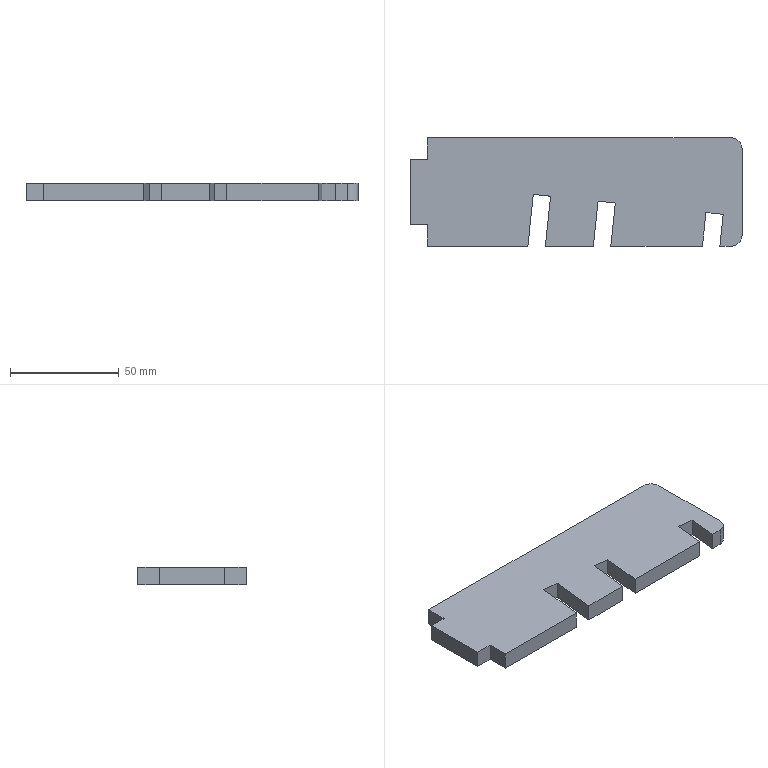Part | SolidWorks | features Fillet 1, FlatPattern 1, SMBaseFlange 1, SheetMetal 1 | 1 solid | 24 faces | box 153 x 50 x 8 mm | volume 56042 mm3 | plane 22 | cylinder 2 | commonest cylinder face diameters 10 x2
STEP:
#1=CARTESIAN_POINT('',(581.248,-4.341,0.));
#2=VERTEX_POINT('',#1);
#3=CARTESIAN_POINT('',(581.248,-14.341,0.));
#4=VERTEX_POINT('',#3);
#5=CARTESIAN_POINT('',(581.248,-4.341,0.));
#6=DIRECTION('',(0.,-1.,0.));
#7=VECTOR('',#6,1000.);
#8=LINE('',#5,#7);
#9=EDGE_CURVE('',#2,#4,#8,.T.);
#10=ORIENTED_EDGE('',*,*,#9,.F.);
#11=CARTESIAN_POINT('',(581.248,-4.341,-8.));
#12=VERTEX_POINT('',#11);
#13=CARTESIAN_POINT('',(581.248,-4.341,-8.));
#14=DIRECTION('',(0.,0.,1.));
#15=VECTOR('',#14,1000.);
#16=LINE('',#13,#15);
#17=EDGE_CURVE('',#12,#2,#16,.T.);
#18=ORIENTED_EDGE('',*,*,#17,.F.);
#19=CARTESIAN_POINT('',(581.248,-14.341,-8.));
#20=VERTEX_POINT('',#19);
#21=CARTESIAN_POINT('',(581.248,-4.341,-8.));
#22=DIRECTION('',(0.,-1.,0.));
#23=VECTOR('',#22,1000.);
#24=LINE('',#21,#23);
#25=EDGE_CURVE('',#12,#20,#24,.T.);
#26=ORIENTED_EDGE('',*,*,#25,.T.);
#27=CARTESIAN_POINT('',(581.248,-14.341,-8.));
#28=DIRECTION('',(0.,0.,1.));
#29=VECTOR('',#28,1000.);
#30=LINE('',#27,#29);
#31=EDGE_CURVE('',#20,#4,#30,.T.);
#32=ORIENTED_EDGE('',*,*,#31,.T.);
#33=EDGE_LOOP('',(#10,#18,#26,#32));
#34=FACE_OUTER_BOUND('',#33,.T.);
#35=CARTESIAN_POINT('',(581.248,-4.341,-8.));
#36=DIRECTION('',(-1.,0.,0.));
#37=DIRECTION('',(0.,0.,1.));
#38=AXIS2_PLACEMENT_3D('',#35,#36,#37);
#39=PLANE('',#38);
#40=ADVANCED_FACE('',(#34),#39,.T.);
#41=CARTESIAN_POINT('',(573.248,-4.341,0.));
#42=VERTEX_POINT('',#41);
#43=CARTESIAN_POINT('',(573.248,-4.341,0.));
#44=DIRECTION('',(1.,0.,0.));
#45=VECTOR('',#44,1000.);
#46=LINE('',#43,#45);
#47=EDGE_CURVE('',#42,#2,#46,.T.);
#48=ORIENTED_EDGE('',*,*,#47,.F.);
#49=CARTESIAN_POINT('',(573.248,-4.341,-8.));
#50=VERTEX_POINT('',#49);
#51=CARTESIAN_POINT('',(573.248,-4.341,-8.));
#52=DIRECTION('',(0.,0.,1.));
#53=VECTOR('',#52,1000.);
#54=LINE('',#51,#53);
#55=EDGE_CURVE('',#50,#42,#54,.T.);
#56=ORIENTED_EDGE('',*,*,#55,.F.);
#57=CARTESIAN_POINT('',(573.248,-4.341,-8.));
#58=DIRECTION('',(1.,0.,0.));
#59=VECTOR('',#58,1000.);
#60=LINE('',#57,#59);
#61=EDGE_CURVE('',#50,#12,#60,.T.);
#62=ORIENTED_EDGE('',*,*,#61,.T.);
#63=ORIENTED_EDGE('',*,*,#17,.T.);
#64=EDGE_LOOP('',(#48,#56,#62,#63));
#65=FACE_OUTER_BOUND('',#64,.T.);
#66=CARTESIAN_POINT('',(573.248,-4.341,-8.));
#67=DIRECTION('',(0.,-1.,0.));
#68=DIRECTION('',(0.,0.,-1.));
#69=AXIS2_PLACEMENT_3D('',#66,#67,#68);
#70=PLANE('',#69);
#71=ADVANCED_FACE('',(#65),#70,.T.);
#72=CARTESIAN_POINT('',(573.248,25.659,0.));
#73=VERTEX_POINT('',#72);
#74=CARTESIAN_POINT('',(573.248,25.659,0.));
#75=DIRECTION('',(0.,-1.,0.));
#76=VECTOR('',#75,1000.);
#77=LINE('',#74,#76);
#78=EDGE_CURVE('',#73,#42,#77,.T.);
#79=ORIENTED_EDGE('',*,*,#78,.F.);
#80=CARTESIAN_POINT('',(573.248,25.659,-8.));
#81=VERTEX_POINT('',#80);
#82=CARTESIAN_POINT('',(573.248,25.659,-8.));
#83=DIRECTION('',(0.,0.,1.));
#84=VECTOR('',#83,1000.);
#85=LINE('',#82,#84);
#86=EDGE_CURVE('',#81,#73,#85,.T.);
#87=ORIENTED_EDGE('',*,*,#86,.F.);
#88=CARTESIAN_POINT('',(573.248,25.659,-8.));
#89=DIRECTION('',(0.,-1.,0.));
#90=VECTOR('',#89,1000.);
#91=LINE('',#88,#90);
#92=EDGE_CURVE('',#81,#50,#91,.T.);
#93=ORIENTED_EDGE('',*,*,#92,.T.);
#94=ORIENTED_EDGE('',*,*,#55,.T.);
#95=EDGE_LOOP('',(#79,#87,#93,#94));
#96=FACE_OUTER_BOUND('',#95,.T.);
#97=CARTESIAN_POINT('',(573.248,25.659,-8.));
#98=DIRECTION('',(-1.,0.,0.));
#99=DIRECTION('',(0.,0.,1.));
#100=AXIS2_PLACEMENT_3D('',#97,#98,#99);
#101=PLANE('',#100);
#102=ADVANCED_FACE('',(#96),#101,.T.);
#103=CARTESIAN_POINT('',(581.248,25.659,0.));
#104=VERTEX_POINT('',#103);
#105=CARTESIAN_POINT('',(581.248,25.659,0.));
#106=DIRECTION('',(-1.,0.,0.));
#107=VECTOR('',#106,1000.);
#108=LINE('',#105,#107);
#109=EDGE_CURVE('',#104,#73,#108,.T.);
#110=ORIENTED_EDGE('',*,*,#109,.F.);
#111=CARTESIAN_POINT('',(581.248,25.659,-8.));
#112=VERTEX_POINT('',#111);
#113=CARTESIAN_POINT('',(581.248,25.659,-8.));
#114=DIRECTION('',(0.,0.,1.));
#115=VECTOR('',#114,1000.);
#116=LINE('',#113,#115);
#117=EDGE_CURVE('',#112,#104,#116,.T.);
#118=ORIENTED_EDGE('',*,*,#117,.F.);
#119=CARTESIAN_POINT('',(581.248,25.659,-8.));
#120=DIRECTION('',(-1.,0.,0.));
#121=VECTOR('',#120,1000.);
#122=LINE('',#119,#121);
#123=EDGE_CURVE('',#112,#81,#122,.T.);
#124=ORIENTED_EDGE('',*,*,#123,.T.);
#125=ORIENTED_EDGE('',*,*,#86,.T.);
#126=EDGE_LOOP('',(#110,#118,#124,#125));
#127=FACE_OUTER_BOUND('',#126,.T.);
#128=CARTESIAN_POINT('',(581.248,25.659,-8.));
#129=DIRECTION('',(0.,1.,0.));
#130=DIRECTION('',(0.,0.,1.));
#131=AXIS2_PLACEMENT_3D('',#128,#129,#130);
#132=PLANE('',#131);
#133=ADVANCED_FACE('',(#127),#132,.T.);
#134=CARTESIAN_POINT('',(581.248,35.659,0.));
#135=VERTEX_POINT('',#134);
#136=CARTESIAN_POINT('',(581.248,35.659,0.));
#137=DIRECTION('',(0.,-1.,0.));
#138=VECTOR('',#137,1000.);
#139=LINE('',#136,#138);
#140=EDGE_CURVE('',#135,#104,#139,.T.);
#141=ORIENTED_EDGE('',*,*,#140,.F.);
#142=CARTESIAN_POINT('',(581.248,35.659,-8.));
#143=VERTEX_POINT('',#142);
#144=CARTESIAN_POINT('',(581.248,35.659,-8.));
#145=DIRECTION('',(0.,0.,1.));
#146=VECTOR('',#145,1000.);
#147=LINE('',#144,#146);
#148=EDGE_CURVE('',#143,#135,#147,.T.);
#149=ORIENTED_EDGE('',*,*,#148,.F.);
#150=CARTESIAN_POINT('',(581.248,35.659,-8.));
#151=DIRECTION('',(0.,-1.,0.));
#152=VECTOR('',#151,1000.);
#153=LINE('',#150,#152);
#154=EDGE_CURVE('',#143,#112,#153,.T.);
#155=ORIENTED_EDGE('',*,*,#154,.T.);
#156=ORIENTED_EDGE('',*,*,#117,.T.);
#157=EDGE_LOOP('',(#141,#149,#155,#156));
#158=FACE_OUTER_BOUND('',#157,.T.);
#159=CARTESIAN_POINT('',(581.248,35.659,-8.));
#160=DIRECTION('',(-1.,0.,0.));
#161=DIRECTION('',(0.,0.,1.));
#162=AXIS2_PLACEMENT_3D('',#159,#160,#161);
#163=PLANE('',#162);
#164=ADVANCED_FACE('',(#158),#163,.T.);
#165=CARTESIAN_POINT('',(721.248,35.659,0.));
#166=VERTEX_POINT('',#165);
#167=CARTESIAN_POINT('',(726.248,35.659,0.));
#168=DIRECTION('',(-1.,0.,0.));
#169=VECTOR('',#168,1000.);
#170=LINE('',#167,#169);
#171=EDGE_CURVE('',#166,#135,#170,.T.);
#172=ORIENTED_EDGE('',*,*,#171,.F.);
#173=CARTESIAN_POINT('',(721.248,35.659,-8.));
#174=VERTEX_POINT('',#173);
#175=CARTESIAN_POINT('',(721.248,35.659,-8.));
#176=DIRECTION('',(0.,0.,-1.));
#177=VECTOR('',#176,1000.);
#178=LINE('',#175,#177);
#179=EDGE_CURVE('',#166,#174,#178,.T.);
#180=ORIENTED_EDGE('',*,*,#179,.T.);
#181=CARTESIAN_POINT('',(726.248,35.659,-8.));
#182=DIRECTION('',(-1.,0.,0.));
#183=VECTOR('',#182,1000.);
#184=LINE('',#181,#183);
#185=EDGE_CURVE('',#174,#143,#184,.T.);
#186=ORIENTED_EDGE('',*,*,#185,.T.);
#187=ORIENTED_EDGE('',*,*,#148,.T.);
#188=EDGE_LOOP('',(#172,#180,#186,#187));
#189=FACE_OUTER_BOUND('',#188,.T.);
#190=CARTESIAN_POINT('',(726.248,35.659,-8.));
#191=DIRECTION('',(0.,1.,0.));
#192=DIRECTION('',(0.,0.,1.));
#193=AXIS2_PLACEMENT_3D('',#190,#191,#192);
#194=PLANE('',#193);
#195=ADVANCED_FACE('',(#189),#194,.T.);
#196=CARTESIAN_POINT('',(726.248,-9.341,0.));
#197=VERTEX_POINT('',#196);
#198=CARTESIAN_POINT('',(726.248,30.659,0.));
#199=VERTEX_POINT('',#198);
#200=CARTESIAN_POINT('',(726.248,-14.341,0.));
#201=DIRECTION('',(0.,1.,0.));
#202=VECTOR('',#201,1000.);
#203=LINE('',#200,#202);
#204=EDGE_CURVE('',#197,#199,#203,.T.);
#205=ORIENTED_EDGE('',*,*,#204,.F.);
#206=CARTESIAN_POINT('',(726.248,-9.341,-8.));
#207=VERTEX_POINT('',#206);
#208=CARTESIAN_POINT('',(726.248,-9.341,-8.));
#209=DIRECTION('',(0.,0.,-1.));
#210=VECTOR('',#209,1000.);
#211=LINE('',#208,#210);
#212=EDGE_CURVE('',#197,#207,#211,.T.);
#213=ORIENTED_EDGE('',*,*,#212,.T.);
#214=CARTESIAN_POINT('',(726.248,30.659,-8.));
#215=VERTEX_POINT('',#214);
#216=CARTESIAN_POINT('',(726.248,-14.341,-8.));
#217=DIRECTION('',(0.,1.,0.));
#218=VECTOR('',#217,1000.);
#219=LINE('',#216,#218);
#220=EDGE_CURVE('',#207,#215,#219,.T.);
#221=ORIENTED_EDGE('',*,*,#220,.T.);
#222=CARTESIAN_POINT('',(726.248,30.659,-8.));
#223=DIRECTION('',(0.,0.,1.));
#224=VECTOR('',#223,1000.);
#225=LINE('',#222,#224);
#226=EDGE_CURVE('',#215,#199,#225,.T.);
#227=ORIENTED_EDGE('',*,*,#226,.T.);
#228=EDGE_LOOP('',(#205,#213,#221,#227));
#229=FACE_OUTER_BOUND('',#228,.T.);
#230=CARTESIAN_POINT('',(726.248,-14.341,-8.));
#231=DIRECTION('',(1.,0.,0.));
#232=DIRECTION('',(0.,0.,-1.));
#233=AXIS2_PLACEMENT_3D('',#230,#231,#232);
#234=PLANE('',#233);
#235=ADVANCED_FACE('',(#229),#234,.T.);
#236=CARTESIAN_POINT('',(716.041,-14.341,-8.));
#237=VERTEX_POINT('',#236);
#238=CARTESIAN_POINT('',(721.248,-14.341,-8.));
#239=VERTEX_POINT('',#238);
#240=CARTESIAN_POINT('',(716.041,-14.341,-8.));
#241=DIRECTION('',(1.,0.,0.));
#242=VECTOR('',#241,1000.);
#243=LINE('',#240,#242);
#244=EDGE_CURVE('',#237,#239,#243,.T.);
#245=ORIENTED_EDGE('',*,*,#244,.T.);
#246=CARTESIAN_POINT('',(721.248,-14.341,0.));
#247=VERTEX_POINT('',#246);
#248=CARTESIAN_POINT('',(721.248,-14.341,-8.));
#249=DIRECTION('',(0.,0.,1.));
#250=VECTOR('',#249,1000.);
#251=LINE('',#248,#250);
#252=EDGE_CURVE('',#239,#247,#251,.T.);
#253=ORIENTED_EDGE('',*,*,#252,.T.);
#254=CARTESIAN_POINT('',(716.041,-14.341,0.));
#255=VERTEX_POINT('',#254);
#256=CARTESIAN_POINT('',(716.041,-14.341,0.));
#257=DIRECTION('',(1.,0.,0.));
#258=VECTOR('',#257,1000.);
#259=LINE('',#256,#258);
#260=EDGE_CURVE('',#255,#247,#259,.T.);
#261=ORIENTED_EDGE('',*,*,#260,.F.);
#262=CARTESIAN_POINT('',(716.041,-14.341,-8.));
#263=DIRECTION('',(0.,0.,1.));
#264=VECTOR('',#263,1000.);
#265=LINE('',#262,#264);
#266=EDGE_CURVE('',#237,#255,#265,.T.);
#267=ORIENTED_EDGE('',*,*,#266,.F.);
#268=EDGE_LOOP('',(#245,#253,#261,#267));
#269=FACE_OUTER_BOUND('',#268,.T.);
#270=CARTESIAN_POINT('',(716.041,-14.341,-8.));
#271=DIRECTION('',(0.,-1.,0.));
#272=DIRECTION('',(0.,0.,-1.));
#273=AXIS2_PLACEMENT_3D('',#270,#271,#272);
#274=PLANE('',#273);
#275=ADVANCED_FACE('',(#269),#274,.T.);
#276=CARTESIAN_POINT('',(717.584,0.3623,0.));
#277=VERTEX_POINT('',#276);
#278=CARTESIAN_POINT('',(717.584,0.3623,0.));
#279=DIRECTION('',(-0.1044,-0.9945,0.));
#280=VECTOR('',#279,1000.);
#281=LINE('',#278,#280);
#282=EDGE_CURVE('',#277,#255,#281,.T.);
#283=ORIENTED_EDGE('',*,*,#282,.F.);
#284=CARTESIAN_POINT('',(717.584,0.3623,-8.));
#285=VERTEX_POINT('',#284);
#286=CARTESIAN_POINT('',(717.584,0.3623,-8.));
#287=DIRECTION('',(0.,0.,1.));
#288=VECTOR('',#287,1000.);
#289=LINE('',#286,#288);
#290=EDGE_CURVE('',#285,#277,#289,.T.);
#291=ORIENTED_EDGE('',*,*,#290,.F.);
#292=CARTESIAN_POINT('',(717.584,0.3623,-8.));
#293=DIRECTION('',(-0.1044,-0.9945,0.));
#294=VECTOR('',#293,1000.);
#295=LINE('',#292,#294);
#296=EDGE_CURVE('',#285,#237,#295,.T.);
#297=ORIENTED_EDGE('',*,*,#296,.T.);
#298=ORIENTED_EDGE('',*,*,#266,.T.);
#299=EDGE_LOOP('',(#283,#291,#297,#298));
#300=FACE_OUTER_BOUND('',#299,.T.);
#301=CARTESIAN_POINT('',(717.584,0.3623,-8.));
#302=DIRECTION('',(-0.9945,0.1044,0.));
#303=DIRECTION('',(-0.1044,-0.9945,0.));
#304=AXIS2_PLACEMENT_3D('',#301,#302,#303);
#305=PLANE('',#304);
#306=ADVANCED_FACE('',(#300),#305,.T.);
#307=CARTESIAN_POINT('',(709.628,1.198,0.));
#308=VERTEX_POINT('',#307);
#309=CARTESIAN_POINT('',(717.584,0.3623,0.));
#310=DIRECTION('',(0.9945,-0.1044,0.));
#311=VECTOR('',#310,1000.);
#312=LINE('',#309,#311);
#313=EDGE_CURVE('',#308,#277,#312,.T.);
#314=ORIENTED_EDGE('',*,*,#313,.F.);
#315=CARTESIAN_POINT('',(709.628,1.198,-8.));
#316=VERTEX_POINT('',#315);
#317=CARTESIAN_POINT('',(709.628,1.198,-8.));
#318=DIRECTION('',(0.,0.,1.));
#319=VECTOR('',#318,1000.);
#320=LINE('',#317,#319);
#321=EDGE_CURVE('',#316,#308,#320,.T.);
#322=ORIENTED_EDGE('',*,*,#321,.F.);
#323=CARTESIAN_POINT('',(717.584,0.3623,-8.));
#324=DIRECTION('',(0.9945,-0.1044,0.));
#325=VECTOR('',#324,1000.);
#326=LINE('',#323,#325);
#327=EDGE_CURVE('',#316,#285,#326,.T.);
#328=ORIENTED_EDGE('',*,*,#327,.T.);
#329=ORIENTED_EDGE('',*,*,#290,.T.);
#330=EDGE_LOOP('',(#314,#322,#328,#329));
#331=FACE_OUTER_BOUND('',#330,.T.);
#332=CARTESIAN_POINT('',(717.584,0.3623,-8.));
#333=DIRECTION('',(-0.1044,-0.9945,0.));
#334=DIRECTION('',(0.9945,-0.1044,0.));
#335=AXIS2_PLACEMENT_3D('',#332,#333,#334);
#336=PLANE('',#335);
#337=ADVANCED_FACE('',(#331),#336,.T.);
#338=CARTESIAN_POINT('',(707.997,-14.341,0.));
#339=VERTEX_POINT('',#338);
#340=CARTESIAN_POINT('',(709.628,1.198,0.));
#341=DIRECTION('',(0.1044,0.9945,0.));
#342=VECTOR('',#341,1000.);
#343=LINE('',#340,#342);
#344=EDGE_CURVE('',#339,#308,#343,.T.);
#345=ORIENTED_EDGE('',*,*,#344,.F.);
#346=CARTESIAN_POINT('',(707.997,-14.341,-8.));
#347=VERTEX_POINT('',#346);
#348=CARTESIAN_POINT('',(707.997,-14.341,-8.));
#349=DIRECTION('',(0.,0.,1.));
#350=VECTOR('',#349,1000.);
#351=LINE('',#348,#350);
#352=EDGE_CURVE('',#347,#339,#351,.T.);
#353=ORIENTED_EDGE('',*,*,#352,.F.);
#354=CARTESIAN_POINT('',(709.628,1.198,-8.));
#355=DIRECTION('',(0.1044,0.9945,0.));
#356=VECTOR('',#355,1000.);
#357=LINE('',#354,#356);
#358=EDGE_CURVE('',#347,#316,#357,.T.);
#359=ORIENTED_EDGE('',*,*,#358,.T.);
#360=ORIENTED_EDGE('',*,*,#321,.T.);
#361=EDGE_LOOP('',(#345,#353,#359,#360));
#362=FACE_OUTER_BOUND('',#361,.T.);
#363=CARTESIAN_POINT('',(709.628,1.198,-8.));
#364=DIRECTION('',(0.9945,-0.1044,0.));
#365=DIRECTION('',(0.1044,0.9945,0.));
#366=AXIS2_PLACEMENT_3D('',#363,#364,#365);
#367=PLANE('',#366);
#368=ADVANCED_FACE('',(#362),#367,.T.);
#369=CARTESIAN_POINT('',(665.766,-14.341,0.));
#370=VERTEX_POINT('',#369);
#371=CARTESIAN_POINT('',(665.766,-14.341,0.));
#372=DIRECTION('',(1.,0.,0.));
#373=VECTOR('',#372,1000.);
#374=LINE('',#371,#373);
#375=EDGE_CURVE('',#370,#339,#374,.T.);
#376=ORIENTED_EDGE('',*,*,#375,.F.);
#377=CARTESIAN_POINT('',(665.766,-14.341,-8.));
#378=VERTEX_POINT('',#377);
#379=CARTESIAN_POINT('',(665.766,-14.341,-8.));
#380=DIRECTION('',(0.,0.,1.));
#381=VECTOR('',#380,1000.);
#382=LINE('',#379,#381);
#383=EDGE_CURVE('',#378,#370,#382,.T.);
#384=ORIENTED_EDGE('',*,*,#383,.F.);
#385=CARTESIAN_POINT('',(665.766,-14.341,-8.));
#386=DIRECTION('',(1.,0.,0.));
#387=VECTOR('',#386,1000.);
#388=LINE('',#385,#387);
#389=EDGE_CURVE('',#378,#347,#388,.T.);
#390=ORIENTED_EDGE('',*,*,#389,.T.);
#391=ORIENTED_EDGE('',*,*,#352,.T.);
#392=EDGE_LOOP('',(#376,#384,#390,#391));
#393=FACE_OUTER_BOUND('',#392,.T.);
#394=CARTESIAN_POINT('',(665.766,-14.341,-8.));
#395=DIRECTION('',(0.,-1.,0.));
#396=DIRECTION('',(1.,0.,0.));
#397=AXIS2_PLACEMENT_3D('',#394,#395,#396);
#398=PLANE('',#397);
#399=ADVANCED_FACE('',(#393),#398,.T.);
#400=CARTESIAN_POINT('',(667.858,5.583,0.));
#401=VERTEX_POINT('',#400);
#402=CARTESIAN_POINT('',(667.858,5.583,0.));
#403=DIRECTION('',(-0.1044,-0.9945,0.));
#404=VECTOR('',#403,1000.);
#405=LINE('',#402,#404);
#406=EDGE_CURVE('',#401,#370,#405,.T.);
#407=ORIENTED_EDGE('',*,*,#406,.F.);
#408=CARTESIAN_POINT('',(667.858,5.583,-8.));
#409=VERTEX_POINT('',#408);
#410=CARTESIAN_POINT('',(667.858,5.583,-8.));
#411=DIRECTION('',(0.,0.,1.));
#412=VECTOR('',#411,1000.);
#413=LINE('',#410,#412);
#414=EDGE_CURVE('',#409,#401,#413,.T.);
#415=ORIENTED_EDGE('',*,*,#414,.F.);
#416=CARTESIAN_POINT('',(667.858,5.583,-8.));
#417=DIRECTION('',(-0.1044,-0.9945,0.));
#418=VECTOR('',#417,1000.);
#419=LINE('',#416,#418);
#420=EDGE_CURVE('',#409,#378,#419,.T.);
#421=ORIENTED_EDGE('',*,*,#420,.T.);
#422=ORIENTED_EDGE('',*,*,#383,.T.);
#423=EDGE_LOOP('',(#407,#415,#421,#422));
#424=FACE_OUTER_BOUND('',#423,.T.);
#425=CARTESIAN_POINT('',(667.858,5.583,-8.));
#426=DIRECTION('',(-0.9945,0.1044,0.));
#427=DIRECTION('',(-0.1044,-0.9945,0.));
#428=AXIS2_PLACEMENT_3D('',#425,#426,#427);
#429=PLANE('',#428);
#430=ADVANCED_FACE('',(#424),#429,.T.);
#431=CARTESIAN_POINT('',(659.901,6.418,0.));
#432=VERTEX_POINT('',#431);
#433=CARTESIAN_POINT('',(667.858,5.583,0.));
#434=DIRECTION('',(0.9945,-0.1044,0.));
#435=VECTOR('',#434,1000.);
#436=LINE('',#433,#435);
#437=EDGE_CURVE('',#432,#401,#436,.T.);
#438=ORIENTED_EDGE('',*,*,#437,.F.);
#439=CARTESIAN_POINT('',(659.901,6.418,-8.));
#440=VERTEX_POINT('',#439);
#441=CARTESIAN_POINT('',(659.901,6.418,-8.));
#442=DIRECTION('',(0.,0.,1.));
#443=VECTOR('',#442,1000.);
#444=LINE('',#441,#443);
#445=EDGE_CURVE('',#440,#432,#444,.T.);
#446=ORIENTED_EDGE('',*,*,#445,.F.);
#447=CARTESIAN_POINT('',(667.858,5.583,-8.));
#448=DIRECTION('',(0.9945,-0.1044,0.));
#449=VECTOR('',#448,1000.);
#450=LINE('',#447,#449);
#451=EDGE_CURVE('',#440,#409,#450,.T.);
#452=ORIENTED_EDGE('',*,*,#451,.T.);
#453=ORIENTED_EDGE('',*,*,#414,.T.);
#454=EDGE_LOOP('',(#438,#446,#452,#453));
#455=FACE_OUTER_BOUND('',#454,.T.);
#456=CARTESIAN_POINT('',(667.858,5.583,-8.));
#457=DIRECTION('',(-0.1044,-0.9945,0.));
#458=DIRECTION('',(0.9945,-0.1044,0.));
#459=AXIS2_PLACEMENT_3D('',#456,#457,#458);
#460=PLANE('',#459);
#461=ADVANCED_FACE('',(#455),#460,.T.);
#462=CARTESIAN_POINT('',(657.722,-14.341,0.));
#463=VERTEX_POINT('',#462);
#464=CARTESIAN_POINT('',(659.901,6.418,0.));
#465=DIRECTION('',(0.1044,0.9945,0.));
#466=VECTOR('',#465,1000.);
#467=LINE('',#464,#466);
#468=EDGE_CURVE('',#463,#432,#467,.T.);
#469=ORIENTED_EDGE('',*,*,#468,.F.);
#470=CARTESIAN_POINT('',(657.722,-14.341,-8.));
#471=VERTEX_POINT('',#470);
#472=CARTESIAN_POINT('',(657.722,-14.341,-8.));
#473=DIRECTION('',(0.,0.,1.));
#474=VECTOR('',#473,1000.);
#475=LINE('',#472,#474);
#476=EDGE_CURVE('',#471,#463,#475,.T.);
#477=ORIENTED_EDGE('',*,*,#476,.F.);
#478=CARTESIAN_POINT('',(659.901,6.418,-8.));
#479=DIRECTION('',(0.1044,0.9945,0.));
#480=VECTOR('',#479,1000.);
#481=LINE('',#478,#480);
#482=EDGE_CURVE('',#471,#440,#481,.T.);
#483=ORIENTED_EDGE('',*,*,#482,.T.);
#484=ORIENTED_EDGE('',*,*,#445,.T.);
#485=EDGE_LOOP('',(#469,#477,#483,#484));
#486=FACE_OUTER_BOUND('',#485,.T.);
#487=CARTESIAN_POINT('',(659.901,6.418,-8.));
#488=DIRECTION('',(0.9945,-0.1044,0.));
#489=DIRECTION('',(0.1044,0.9945,0.));
#490=AXIS2_PLACEMENT_3D('',#487,#488,#489);
#491=PLANE('',#490);
#492=ADVANCED_FACE('',(#486),#491,.T.);
#493=CARTESIAN_POINT('',(635.601,-14.341,0.));
#494=VERTEX_POINT('',#493);
#495=CARTESIAN_POINT('',(635.601,-14.341,0.));
#496=DIRECTION('',(1.,0.,0.));
#497=VECTOR('',#496,1000.);
#498=LINE('',#495,#497);
#499=EDGE_CURVE('',#494,#463,#498,.T.);
#500=ORIENTED_EDGE('',*,*,#499,.F.);
#501=CARTESIAN_POINT('',(635.601,-14.341,-8.));
#502=VERTEX_POINT('',#501);
#503=CARTESIAN_POINT('',(635.601,-14.341,-8.));
#504=DIRECTION('',(0.,0.,1.));
#505=VECTOR('',#504,1000.);
#506=LINE('',#503,#505);
#507=EDGE_CURVE('',#502,#494,#506,.T.);
#508=ORIENTED_EDGE('',*,*,#507,.F.);
#509=CARTESIAN_POINT('',(635.601,-14.341,-8.));
#510=DIRECTION('',(1.,0.,0.));
#511=VECTOR('',#510,1000.);
#512=LINE('',#509,#511);
#513=EDGE_CURVE('',#502,#471,#512,.T.);
#514=ORIENTED_EDGE('',*,*,#513,.T.);
#515=ORIENTED_EDGE('',*,*,#476,.T.);
#516=EDGE_LOOP('',(#500,#508,#514,#515));
#517=FACE_OUTER_BOUND('',#516,.T.);
#518=CARTESIAN_POINT('',(635.601,-14.341,-8.));
#519=DIRECTION('',(0.,-1.,0.));
#520=DIRECTION('',(0.,0.,-1.));
#521=AXIS2_PLACEMENT_3D('',#518,#519,#520);
#522=PLANE('',#521);
#523=ADVANCED_FACE('',(#517),#522,.T.);
#524=CARTESIAN_POINT('',(638.022,8.715,0.));
#525=VERTEX_POINT('',#524);
#526=CARTESIAN_POINT('',(638.022,8.715,0.));
#527=DIRECTION('',(-0.1044,-0.9945,0.));
#528=VECTOR('',#527,1000.);
#529=LINE('',#526,#528);
#530=EDGE_CURVE('',#525,#494,#529,.T.);
#531=ORIENTED_EDGE('',*,*,#530,.F.);
#532=CARTESIAN_POINT('',(638.022,8.715,-8.));
#533=VERTEX_POINT('',#532);
#534=CARTESIAN_POINT('',(638.022,8.715,-8.));
#535=DIRECTION('',(0.,0.,1.));
#536=VECTOR('',#535,1000.);
#537=LINE('',#534,#536);
#538=EDGE_CURVE('',#533,#525,#537,.T.);
#539=ORIENTED_EDGE('',*,*,#538,.F.);
#540=CARTESIAN_POINT('',(638.022,8.715,-8.));
#541=DIRECTION('',(-0.1044,-0.9945,0.));
#542=VECTOR('',#541,1000.);
#543=LINE('',#540,#542);
#544=EDGE_CURVE('',#533,#502,#543,.T.);
#545=ORIENTED_EDGE('',*,*,#544,.T.);
#546=ORIENTED_EDGE('',*,*,#507,.T.);
#547=EDGE_LOOP('',(#531,#539,#545,#546));
#548=FACE_OUTER_BOUND('',#547,.T.);
#549=CARTESIAN_POINT('',(638.022,8.715,-8.));
#550=DIRECTION('',(-0.9945,0.1044,0.));
#551=DIRECTION('',(-0.1044,-0.9945,0.));
#552=AXIS2_PLACEMENT_3D('',#549,#550,#551);
#553=PLANE('',#552);
#554=ADVANCED_FACE('',(#548),#553,.T.);
#555=CARTESIAN_POINT('',(630.065,9.551,0.));
#556=VERTEX_POINT('',#555);
#557=CARTESIAN_POINT('',(638.022,8.715,0.));
#558=DIRECTION('',(0.9945,-0.1044,0.));
#559=VECTOR('',#558,1000.);
#560=LINE('',#557,#559);
#561=EDGE_CURVE('',#556,#525,#560,.T.);
#562=ORIENTED_EDGE('',*,*,#561,.F.);
#563=CARTESIAN_POINT('',(630.065,9.551,-8.));
#564=VERTEX_POINT('',#563);
#565=CARTESIAN_POINT('',(630.065,9.551,-8.));
#566=DIRECTION('',(0.,0.,1.));
#567=VECTOR('',#566,1000.);
#568=LINE('',#565,#567);
#569=EDGE_CURVE('',#564,#556,#568,.T.);
#570=ORIENTED_EDGE('',*,*,#569,.F.);
#571=CARTESIAN_POINT('',(638.022,8.715,-8.));
#572=DIRECTION('',(0.9945,-0.1044,0.));
#573=VECTOR('',#572,1000.);
#574=LINE('',#571,#573);
#575=EDGE_CURVE('',#564,#533,#574,.T.);
#576=ORIENTED_EDGE('',*,*,#575,.T.);
#577=ORIENTED_EDGE('',*,*,#538,.T.);
#578=EDGE_LOOP('',(#562,#570,#576,#577));
#579=FACE_OUTER_BOUND('',#578,.T.);
#580=CARTESIAN_POINT('',(638.022,8.715,-8.));
#581=DIRECTION('',(-0.1044,-0.9945,0.));
#582=DIRECTION('',(0.9945,-0.1044,0.));
#583=AXIS2_PLACEMENT_3D('',#580,#581,#582);
#584=PLANE('',#583);
#585=ADVANCED_FACE('',(#579),#584,.T.);
#586=CARTESIAN_POINT('',(627.557,-14.341,0.));
#587=VERTEX_POINT('',#586);
#588=CARTESIAN_POINT('',(630.065,9.551,0.));
#589=DIRECTION('',(0.1044,0.9945,0.));
#590=VECTOR('',#589,1000.);
#591=LINE('',#588,#590);
#592=EDGE_CURVE('',#587,#556,#591,.T.);
#593=ORIENTED_EDGE('',*,*,#592,.F.);
#594=CARTESIAN_POINT('',(627.557,-14.341,-8.));
#595=VERTEX_POINT('',#594);
#596=CARTESIAN_POINT('',(627.557,-14.341,-8.));
#597=DIRECTION('',(0.,0.,1.));
#598=VECTOR('',#597,1000.);
#599=LINE('',#596,#598);
#600=EDGE_CURVE('',#595,#587,#599,.T.);
#601=ORIENTED_EDGE('',*,*,#600,.F.);
#602=CARTESIAN_POINT('',(630.065,9.551,-8.));
#603=DIRECTION('',(0.1044,0.9945,0.));
#604=VECTOR('',#603,1000.);
#605=LINE('',#602,#604);
#606=EDGE_CURVE('',#595,#564,#605,.T.);
#607=ORIENTED_EDGE('',*,*,#606,.T.);
#608=ORIENTED_EDGE('',*,*,#569,.T.);
#609=EDGE_LOOP('',(#593,#601,#607,#608));
#610=FACE_OUTER_BOUND('',#609,.T.);
#611=CARTESIAN_POINT('',(630.065,9.551,-8.));
#612=DIRECTION('',(0.9945,-0.1044,0.));
#613=DIRECTION('',(0.1044,0.9945,0.));
#614=AXIS2_PLACEMENT_3D('',#611,#612,#613);
#615=PLANE('',#614);
#616=ADVANCED_FACE('',(#610),#615,.T.);
#617=CARTESIAN_POINT('',(581.248,-14.341,0.));
#618=DIRECTION('',(1.,0.,0.));
#619=VECTOR('',#618,1000.);
#620=LINE('',#617,#619);
#621=EDGE_CURVE('',#4,#587,#620,.T.);
#622=ORIENTED_EDGE('',*,*,#621,.F.);
#623=ORIENTED_EDGE('',*,*,#31,.F.);
#624=CARTESIAN_POINT('',(581.248,-14.341,-8.));
#625=DIRECTION('',(1.,0.,0.));
#626=VECTOR('',#625,1000.);
#627=LINE('',#624,#626);
#628=EDGE_CURVE('',#20,#595,#627,.T.);
#629=ORIENTED_EDGE('',*,*,#628,.T.);
#630=ORIENTED_EDGE('',*,*,#600,.T.);
#631=EDGE_LOOP('',(#622,#623,#629,#630));
#632=FACE_OUTER_BOUND('',#631,.T.);
#633=CARTESIAN_POINT('',(581.248,-14.341,-8.));
#634=DIRECTION('',(0.,-1.,0.));
#635=DIRECTION('',(1.,0.,0.));
#636=AXIS2_PLACEMENT_3D('',#633,#634,#635);
#637=PLANE('',#636);
#638=ADVANCED_FACE('',(#632),#637,.T.);
#639=ORIENTED_EDGE('',*,*,#220,.F.);
#640=CARTESIAN_POINT('',(721.248,-9.341,-8.));
#641=DIRECTION('',(0.,0.,-1.));
#642=DIRECTION('',(1.,0.,0.));
#643=AXIS2_PLACEMENT_3D('',#640,#641,#642);
#644=CIRCLE('',#643,5.);
#645=EDGE_CURVE('',#207,#239,#644,.T.);
#646=ORIENTED_EDGE('',*,*,#645,.T.);
#647=ORIENTED_EDGE('',*,*,#244,.F.);
#648=ORIENTED_EDGE('',*,*,#296,.F.);
#649=ORIENTED_EDGE('',*,*,#327,.F.);
#650=ORIENTED_EDGE('',*,*,#358,.F.);
#651=ORIENTED_EDGE('',*,*,#389,.F.);
#652=ORIENTED_EDGE('',*,*,#420,.F.);
#653=ORIENTED_EDGE('',*,*,#451,.F.);
#654=ORIENTED_EDGE('',*,*,#482,.F.);
#655=ORIENTED_EDGE('',*,*,#513,.F.);
#656=ORIENTED_EDGE('',*,*,#544,.F.);
#657=ORIENTED_EDGE('',*,*,#575,.F.);
#658=ORIENTED_EDGE('',*,*,#606,.F.);
#659=ORIENTED_EDGE('',*,*,#628,.F.);
#660=ORIENTED_EDGE('',*,*,#25,.F.);
#661=ORIENTED_EDGE('',*,*,#61,.F.);
#662=ORIENTED_EDGE('',*,*,#92,.F.);
#663=ORIENTED_EDGE('',*,*,#123,.F.);
#664=ORIENTED_EDGE('',*,*,#154,.F.);
#665=ORIENTED_EDGE('',*,*,#185,.F.);
#666=CARTESIAN_POINT('',(721.248,30.659,-8.));
#667=DIRECTION('',(0.,0.,-1.));
#668=DIRECTION('',(1.,0.,0.));
#669=AXIS2_PLACEMENT_3D('',#666,#667,#668);
#670=CIRCLE('',#669,5.);
#671=EDGE_CURVE('',#174,#215,#670,.T.);
#672=ORIENTED_EDGE('',*,*,#671,.T.);
#673=EDGE_LOOP('',(#639,#646,#647,#648,#649,#650,#651,#652,#653,#654,#655,#656,#657,#658,#659,#660,#661,#662,#663,#664,#665,#672));
#674=FACE_OUTER_BOUND('',#673,.T.);
#675=CARTESIAN_POINT('',(0.,0.,-8.));
#676=DIRECTION('',(0.,0.,1.));
#677=DIRECTION('',(1.,0.,0.));
#678=AXIS2_PLACEMENT_3D('',#675,#676,#677);
#679=PLANE('',#678);
#680=ADVANCED_FACE('',(#674),#679,.F.);
#681=ORIENTED_EDGE('',*,*,#260,.T.);
#682=CARTESIAN_POINT('',(721.248,-9.341,0.));
#683=DIRECTION('',(0.,0.,1.));
#684=DIRECTION('',(1.,0.,0.));
#685=AXIS2_PLACEMENT_3D('',#682,#683,#684);
#686=CIRCLE('',#685,5.);
#687=EDGE_CURVE('',#247,#197,#686,.T.);
#688=ORIENTED_EDGE('',*,*,#687,.T.);
#689=ORIENTED_EDGE('',*,*,#204,.T.);
#690=CARTESIAN_POINT('',(721.248,30.659,0.));
#691=DIRECTION('',(0.,0.,1.));
#692=DIRECTION('',(1.,0.,0.));
#693=AXIS2_PLACEMENT_3D('',#690,#691,#692);
#694=CIRCLE('',#693,5.);
#695=EDGE_CURVE('',#199,#166,#694,.T.);
#696=ORIENTED_EDGE('',*,*,#695,.T.);
#697=ORIENTED_EDGE('',*,*,#171,.T.);
#698=ORIENTED_EDGE('',*,*,#140,.T.);
#699=ORIENTED_EDGE('',*,*,#109,.T.);
#700=ORIENTED_EDGE('',*,*,#78,.T.);
#701=ORIENTED_EDGE('',*,*,#47,.T.);
#702=ORIENTED_EDGE('',*,*,#9,.T.);
#703=ORIENTED_EDGE('',*,*,#621,.T.);
#704=ORIENTED_EDGE('',*,*,#592,.T.);
#705=ORIENTED_EDGE('',*,*,#561,.T.);
#706=ORIENTED_EDGE('',*,*,#530,.T.);
#707=ORIENTED_EDGE('',*,*,#499,.T.);
#708=ORIENTED_EDGE('',*,*,#468,.T.);
#709=ORIENTED_EDGE('',*,*,#437,.T.);
#710=ORIENTED_EDGE('',*,*,#406,.T.);
#711=ORIENTED_EDGE('',*,*,#375,.T.);
#712=ORIENTED_EDGE('',*,*,#344,.T.);
#713=ORIENTED_EDGE('',*,*,#313,.T.);
#714=ORIENTED_EDGE('',*,*,#282,.T.);
#715=EDGE_LOOP('',(#681,#688,#689,#696,#697,#698,#699,#700,#701,#702,#703,#704,#705,#706,#707,#708,#709,#710,#711,#712,#713,#714));
#716=FACE_OUTER_BOUND('',#715,.T.);
#717=CARTESIAN_POINT('',(0.,0.,0.));
#718=DIRECTION('',(0.,0.,1.));
#719=DIRECTION('',(1.,0.,0.));
#720=AXIS2_PLACEMENT_3D('',#717,#718,#719);
#721=PLANE('',#720);
#722=ADVANCED_FACE('',(#716),#721,.T.);
#723=ORIENTED_EDGE('',*,*,#645,.F.);
#724=ORIENTED_EDGE('',*,*,#212,.F.);
#725=ORIENTED_EDGE('',*,*,#687,.F.);
#726=ORIENTED_EDGE('',*,*,#252,.F.);
#727=EDGE_LOOP('',(#723,#724,#725,#726));
#728=FACE_OUTER_BOUND('',#727,.T.);
#729=CARTESIAN_POINT('',(721.248,-9.341,-8.));
#730=DIRECTION('',(0.,0.,1.));
#731=DIRECTION('',(1.,0.,0.));
#732=AXIS2_PLACEMENT_3D('',#729,#730,#731);
#733=CYLINDRICAL_SURFACE('',#732,5.);
#734=ADVANCED_FACE('',(#728),#733,.T.);
#735=ORIENTED_EDGE('',*,*,#671,.F.);
#736=ORIENTED_EDGE('',*,*,#179,.F.);
#737=ORIENTED_EDGE('',*,*,#695,.F.);
#738=ORIENTED_EDGE('',*,*,#226,.F.);
#739=EDGE_LOOP('',(#735,#736,#737,#738));
#740=FACE_OUTER_BOUND('',#739,.T.);
#741=CARTESIAN_POINT('',(721.248,30.659,-8.));
#742=DIRECTION('',(0.,0.,1.));
#743=DIRECTION('',(1.,0.,0.));
#744=AXIS2_PLACEMENT_3D('',#741,#742,#743);
#745=CYLINDRICAL_SURFACE('',#744,5.);
#746=ADVANCED_FACE('',(#740),#745,.T.);
#747=CLOSED_SHELL('',(#40,#71,#102,#133,#164,#195,#235,#275,#306,#337,#368,#399,#430,#461,#492,#523,#554,#585,#616,#638,#680,#722,#734,#746));
#748=MANIFOLD_SOLID_BREP('',#747);
#749=CARTESIAN_POINT('',(0.,0.,0.));
#750=DIRECTION('',(0.,0.,1.));
#751=DIRECTION('',(1.,0.,0.));
#752=AXIS2_PLACEMENT_3D('',#749,#750,#751);
#753=(LENGTH_UNIT()NAMED_UNIT(*)SI_UNIT(.MILLI.,.METRE.));
#754=UNCERTAINTY_MEASURE_WITH_UNIT(LENGTH_MEASURE(0.00001),#753,'','');
#755=(NAMED_UNIT(*)PLANE_ANGLE_UNIT()SI_UNIT($,.RADIAN.));
#756=(NAMED_UNIT(*)SI_UNIT($,.STERADIAN.)SOLID_ANGLE_UNIT());
#757=(GEOMETRIC_REPRESENTATION_CONTEXT(3)GLOBAL_UNCERTAINTY_ASSIGNED_CONTEXT((#754))GLOBAL_UNIT_ASSIGNED_CONTEXT((#753,#755,#756))REPRESENTATION_CONTEXT('',''));
#758=ADVANCED_BREP_SHAPE_REPRESENTATION('',(#748,#752),#757);